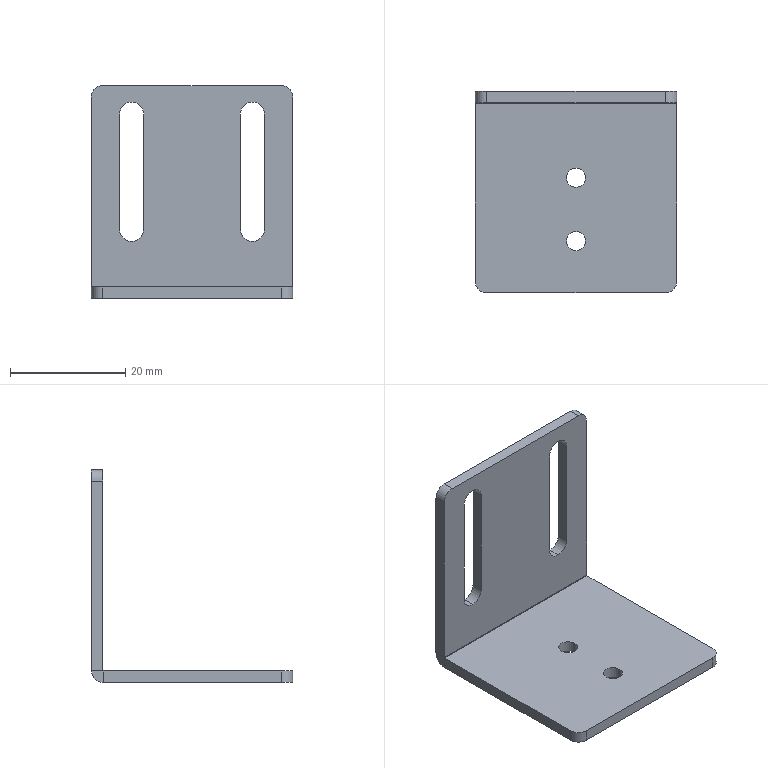Part | STEP file | Cable carrier adapter plate 2 | 1 solid | 32 faces | box 35 x 35 x 37 mm | volume 4434 mm3 | cylinder 16 | plane 16 | commonest cylinder face diameters 4.2 x7 3.3 x4 4 x4 0.2 x1